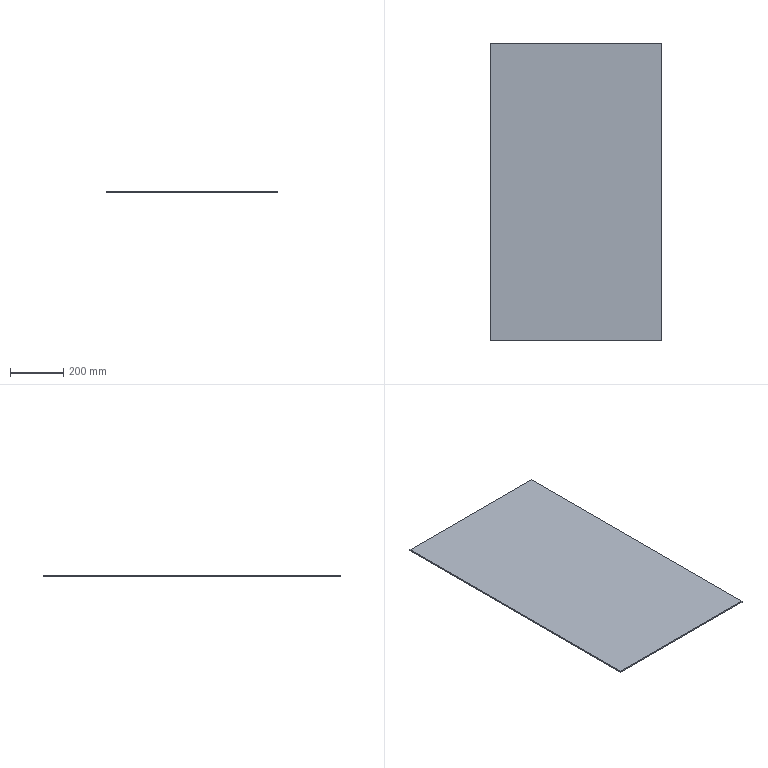Part | SolidWorks | features Extrusion 1 | 1 solid | 6 faces | box 646 x 1119 x 5 mm | volume 3614370 mm3 | plane 6
STEP:
#1=CARTESIAN_POINT('',(323.,-559.5,0.));
#2=VERTEX_POINT('',#1);
#3=CARTESIAN_POINT('',(323.,559.5,0.));
#4=VERTEX_POINT('',#3);
#5=CARTESIAN_POINT('',(323.,559.5,0.));
#6=DIRECTION('',(0.,1.,0.));
#7=VECTOR('',#6,1000.);
#8=LINE('',#5,#7);
#9=EDGE_CURVE('',#2,#4,#8,.T.);
#10=ORIENTED_EDGE('',*,*,#9,.T.);
#11=CARTESIAN_POINT('',(323.,559.5,5.));
#12=VERTEX_POINT('',#11);
#13=CARTESIAN_POINT('',(323.,559.5,5.));
#14=DIRECTION('',(0.,0.,-1.));
#15=VECTOR('',#14,1000.);
#16=LINE('',#13,#15);
#17=EDGE_CURVE('',#12,#4,#16,.T.);
#18=ORIENTED_EDGE('',*,*,#17,.F.);
#19=CARTESIAN_POINT('',(323.,-559.5,5.));
#20=VERTEX_POINT('',#19);
#21=CARTESIAN_POINT('',(323.,559.5,5.));
#22=DIRECTION('',(0.,1.,0.));
#23=VECTOR('',#22,1000.);
#24=LINE('',#21,#23);
#25=EDGE_CURVE('',#20,#12,#24,.T.);
#26=ORIENTED_EDGE('',*,*,#25,.F.);
#27=CARTESIAN_POINT('',(323.,-559.5,5.));
#28=DIRECTION('',(0.,0.,-1.));
#29=VECTOR('',#28,1000.);
#30=LINE('',#27,#29);
#31=EDGE_CURVE('',#20,#2,#30,.T.);
#32=ORIENTED_EDGE('',*,*,#31,.T.);
#33=EDGE_LOOP('',(#10,#18,#26,#32));
#34=FACE_OUTER_BOUND('',#33,.T.);
#35=CARTESIAN_POINT('',(323.,559.5,5.));
#36=DIRECTION('',(-1.,0.,0.));
#37=DIRECTION('',(0.,-1.,0.));
#38=AXIS2_PLACEMENT_3D('',#35,#36,#37);
#39=PLANE('',#38);
#40=ADVANCED_FACE('',(#34),#39,.F.);
#41=CARTESIAN_POINT('',(-323.,559.5,0.));
#42=VERTEX_POINT('',#41);
#43=CARTESIAN_POINT('',(-323.,559.5,0.));
#44=DIRECTION('',(-1.,0.,0.));
#45=VECTOR('',#44,1000.);
#46=LINE('',#43,#45);
#47=EDGE_CURVE('',#4,#42,#46,.T.);
#48=ORIENTED_EDGE('',*,*,#47,.T.);
#49=CARTESIAN_POINT('',(-323.,559.5,5.));
#50=VERTEX_POINT('',#49);
#51=CARTESIAN_POINT('',(-323.,559.5,5.));
#52=DIRECTION('',(0.,0.,-1.));
#53=VECTOR('',#52,1000.);
#54=LINE('',#51,#53);
#55=EDGE_CURVE('',#50,#42,#54,.T.);
#56=ORIENTED_EDGE('',*,*,#55,.F.);
#57=CARTESIAN_POINT('',(-323.,559.5,5.));
#58=DIRECTION('',(-1.,0.,0.));
#59=VECTOR('',#58,1000.);
#60=LINE('',#57,#59);
#61=EDGE_CURVE('',#12,#50,#60,.T.);
#62=ORIENTED_EDGE('',*,*,#61,.F.);
#63=ORIENTED_EDGE('',*,*,#17,.T.);
#64=EDGE_LOOP('',(#48,#56,#62,#63));
#65=FACE_OUTER_BOUND('',#64,.T.);
#66=CARTESIAN_POINT('',(-323.,559.5,5.));
#67=DIRECTION('',(0.,-1.,0.));
#68=DIRECTION('',(0.,0.,-1.));
#69=AXIS2_PLACEMENT_3D('',#66,#67,#68);
#70=PLANE('',#69);
#71=ADVANCED_FACE('',(#65),#70,.F.);
#72=CARTESIAN_POINT('',(-323.,-559.5,0.));
#73=VERTEX_POINT('',#72);
#74=CARTESIAN_POINT('',(-323.,559.5,0.));
#75=DIRECTION('',(0.,-1.,0.));
#76=VECTOR('',#75,1000.);
#77=LINE('',#74,#76);
#78=EDGE_CURVE('',#42,#73,#77,.T.);
#79=ORIENTED_EDGE('',*,*,#78,.T.);
#80=CARTESIAN_POINT('',(-323.,-559.5,5.));
#81=VERTEX_POINT('',#80);
#82=CARTESIAN_POINT('',(-323.,-559.5,5.));
#83=DIRECTION('',(0.,0.,-1.));
#84=VECTOR('',#83,1000.);
#85=LINE('',#82,#84);
#86=EDGE_CURVE('',#81,#73,#85,.T.);
#87=ORIENTED_EDGE('',*,*,#86,.F.);
#88=CARTESIAN_POINT('',(-323.,559.5,5.));
#89=DIRECTION('',(0.,-1.,0.));
#90=VECTOR('',#89,1000.);
#91=LINE('',#88,#90);
#92=EDGE_CURVE('',#50,#81,#91,.T.);
#93=ORIENTED_EDGE('',*,*,#92,.F.);
#94=ORIENTED_EDGE('',*,*,#55,.T.);
#95=EDGE_LOOP('',(#79,#87,#93,#94));
#96=FACE_OUTER_BOUND('',#95,.T.);
#97=CARTESIAN_POINT('',(-323.,559.5,5.));
#98=DIRECTION('',(1.,0.,0.));
#99=DIRECTION('',(0.,1.,0.));
#100=AXIS2_PLACEMENT_3D('',#97,#98,#99);
#101=PLANE('',#100);
#102=ADVANCED_FACE('',(#96),#101,.F.);
#103=CARTESIAN_POINT('',(-323.,-559.5,0.));
#104=DIRECTION('',(1.,0.,0.));
#105=VECTOR('',#104,1000.);
#106=LINE('',#103,#105);
#107=EDGE_CURVE('',#73,#2,#106,.T.);
#108=ORIENTED_EDGE('',*,*,#107,.T.);
#109=ORIENTED_EDGE('',*,*,#31,.F.);
#110=CARTESIAN_POINT('',(-323.,-559.5,5.));
#111=DIRECTION('',(1.,0.,0.));
#112=VECTOR('',#111,1000.);
#113=LINE('',#110,#112);
#114=EDGE_CURVE('',#81,#20,#113,.T.);
#115=ORIENTED_EDGE('',*,*,#114,.F.);
#116=ORIENTED_EDGE('',*,*,#86,.T.);
#117=EDGE_LOOP('',(#108,#109,#115,#116));
#118=FACE_OUTER_BOUND('',#117,.T.);
#119=CARTESIAN_POINT('',(-323.,-559.5,5.));
#120=DIRECTION('',(0.,1.,0.));
#121=DIRECTION('',(0.,0.,1.));
#122=AXIS2_PLACEMENT_3D('',#119,#120,#121);
#123=PLANE('',#122);
#124=ADVANCED_FACE('',(#118),#123,.F.);
#125=ORIENTED_EDGE('',*,*,#25,.T.);
#126=ORIENTED_EDGE('',*,*,#61,.T.);
#127=ORIENTED_EDGE('',*,*,#92,.T.);
#128=ORIENTED_EDGE('',*,*,#114,.T.);
#129=EDGE_LOOP('',(#125,#126,#127,#128));
#130=FACE_OUTER_BOUND('',#129,.T.);
#131=CARTESIAN_POINT('',(0.,0.,5.));
#132=DIRECTION('',(0.,0.,1.));
#133=DIRECTION('',(1.,0.,0.));
#134=AXIS2_PLACEMENT_3D('',#131,#132,#133);
#135=PLANE('',#134);
#136=ADVANCED_FACE('',(#130),#135,.T.);
#137=ORIENTED_EDGE('',*,*,#9,.F.);
#138=ORIENTED_EDGE('',*,*,#107,.F.);
#139=ORIENTED_EDGE('',*,*,#78,.F.);
#140=ORIENTED_EDGE('',*,*,#47,.F.);
#141=EDGE_LOOP('',(#137,#138,#139,#140));
#142=FACE_OUTER_BOUND('',#141,.T.);
#143=CARTESIAN_POINT('',(0.,0.,0.));
#144=DIRECTION('',(0.,0.,1.));
#145=DIRECTION('',(1.,0.,0.));
#146=AXIS2_PLACEMENT_3D('',#143,#144,#145);
#147=PLANE('',#146);
#148=ADVANCED_FACE('',(#142),#147,.F.);
#149=CLOSED_SHELL('',(#40,#71,#102,#124,#136,#148));
#150=MANIFOLD_SOLID_BREP('',#149);
#151=CARTESIAN_POINT('',(0.,0.,0.));
#152=DIRECTION('',(0.,0.,1.));
#153=DIRECTION('',(1.,0.,0.));
#154=AXIS2_PLACEMENT_3D('',#151,#152,#153);
#155=(LENGTH_UNIT()NAMED_UNIT(*)SI_UNIT(.MILLI.,.METRE.));
#156=UNCERTAINTY_MEASURE_WITH_UNIT(LENGTH_MEASURE(0.00001),#155,'','');
#157=(NAMED_UNIT(*)PLANE_ANGLE_UNIT()SI_UNIT($,.RADIAN.));
#158=(NAMED_UNIT(*)SI_UNIT($,.STERADIAN.)SOLID_ANGLE_UNIT());
#159=(GEOMETRIC_REPRESENTATION_CONTEXT(3)GLOBAL_UNCERTAINTY_ASSIGNED_CONTEXT((#156))GLOBAL_UNIT_ASSIGNED_CONTEXT((#155,#157,#158))REPRESENTATION_CONTEXT('',''));
#160=ADVANCED_BREP_SHAPE_REPRESENTATION('',(#150,#154),#159);